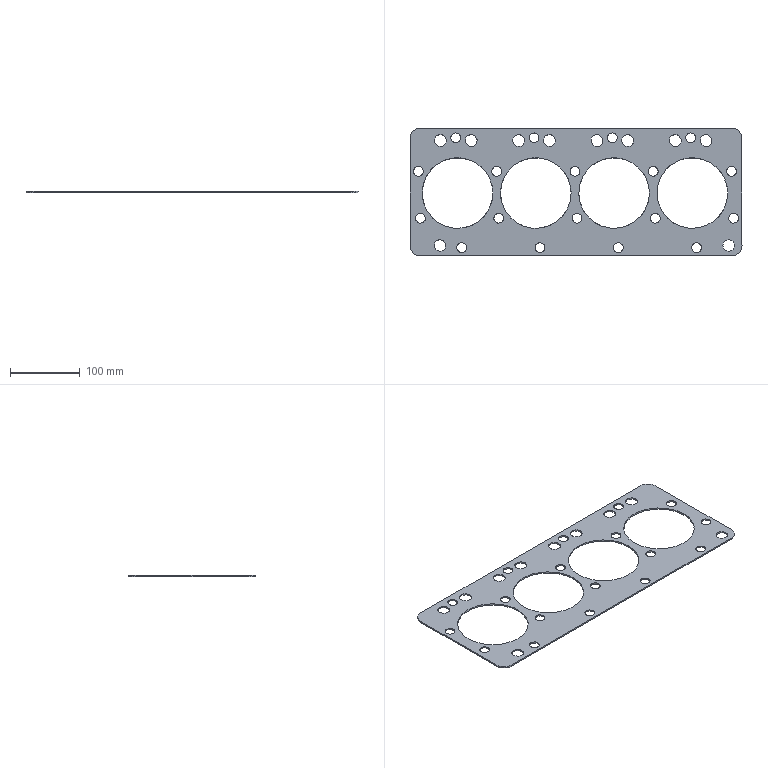Part | SolidWorks | features BaseBody 1 | 1 solid | 139 faces | box 475 x 183 x 2 mm | volume 99346 mm3 | cylinder 133 | plane 6 | commonest cylinder face diameters 13.999 x53 17 x32 14 x18 100.998 x12 16.5 x8 30 x6